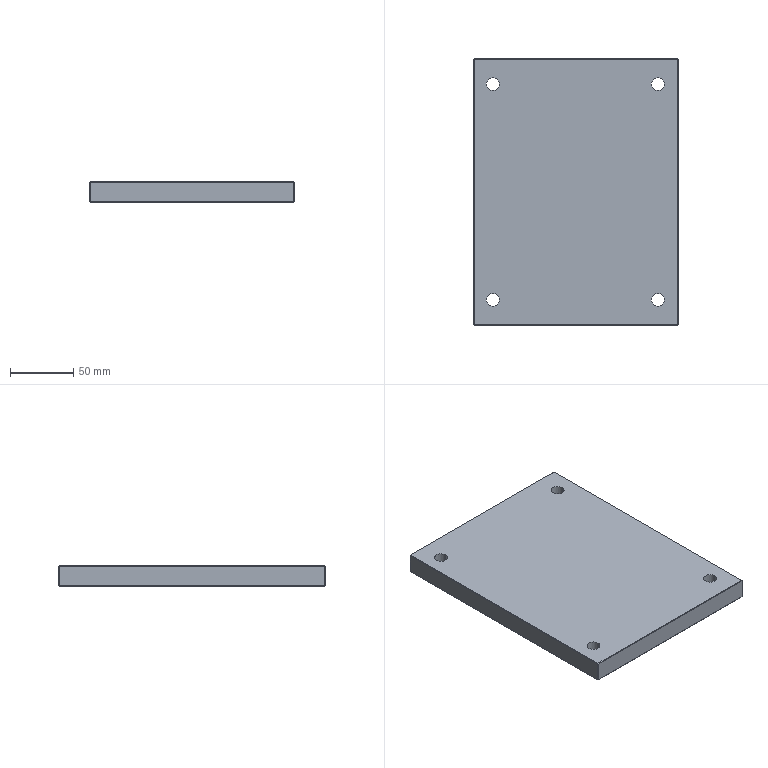Part | SolidWorks | features BaseBody 1 | 1 solid | 34 faces | box 161 x 210 x 16 mm | volume 535538 mm3 | plane 26 | cylinder 8 | commonest cylinder face diameters 10.2 x8
STEP:
#1=CARTESIAN_POINT('',(-15.1,290.,331.));
#2=VERTEX_POINT('',#1);
#3=CARTESIAN_POINT('',(-4.9,290.,331.));
#4=VERTEX_POINT('',#3);
#5=CARTESIAN_POINT('',(-10.,290.,331.));
#6=DIRECTION('',(0.,0.,1.));
#7=DIRECTION('',(0.,-1.,0.));
#8=AXIS2_PLACEMENT_3D('',#5,#6,#7);
#9=CIRCLE('',#8,5.1);
#10=EDGE_CURVE('',#2,#4,#9,.T.);
#11=ORIENTED_EDGE('',*,*,#10,.T.);
#12=CARTESIAN_POINT('',(-4.9,290.,315.));
#13=VERTEX_POINT('',#12);
#14=CARTESIAN_POINT('',(-4.9,290.,315.));
#15=DIRECTION('',(0.,0.,-1.));
#16=VECTOR('',#15,1000.);
#17=LINE('',#14,#16);
#18=EDGE_CURVE('',#4,#13,#17,.T.);
#19=ORIENTED_EDGE('',*,*,#18,.T.);
#20=CARTESIAN_POINT('',(-15.1,290.,315.));
#21=VERTEX_POINT('',#20);
#22=CARTESIAN_POINT('',(-10.,290.,315.));
#23=DIRECTION('',(0.,0.,-1.));
#24=DIRECTION('',(-1.,0.,0.));
#25=AXIS2_PLACEMENT_3D('',#22,#23,#24);
#26=CIRCLE('',#25,5.1);
#27=EDGE_CURVE('',#13,#21,#26,.T.);
#28=ORIENTED_EDGE('',*,*,#27,.T.);
#29=CARTESIAN_POINT('',(-15.1,290.,315.));
#30=DIRECTION('',(0.,0.,-1.));
#31=VECTOR('',#30,1000.);
#32=LINE('',#29,#31);
#33=EDGE_CURVE('',#2,#21,#32,.T.);
#34=ORIENTED_EDGE('',*,*,#33,.F.);
#35=EDGE_LOOP('',(#11,#19,#28,#34));
#36=FACE_OUTER_BOUND('',#35,.T.);
#37=CARTESIAN_POINT('',(-10.,290.,315.));
#38=DIRECTION('',(0.,0.,-1.));
#39=DIRECTION('',(-1.,0.,0.));
#40=AXIS2_PLACEMENT_3D('',#37,#38,#39);
#41=CYLINDRICAL_SURFACE('',#40,5.1);
#42=ADVANCED_FACE('',(#36),#41,.F.);
#43=CARTESIAN_POINT('',(-15.1,460.,331.));
#44=VERTEX_POINT('',#43);
#45=CARTESIAN_POINT('',(-4.9,460.,331.));
#46=VERTEX_POINT('',#45);
#47=CARTESIAN_POINT('',(-10.,460.,331.));
#48=DIRECTION('',(0.,0.,1.));
#49=DIRECTION('',(0.,-1.,0.));
#50=AXIS2_PLACEMENT_3D('',#47,#48,#49);
#51=CIRCLE('',#50,5.1);
#52=EDGE_CURVE('',#44,#46,#51,.T.);
#53=ORIENTED_EDGE('',*,*,#52,.T.);
#54=CARTESIAN_POINT('',(-4.9,460.,315.));
#55=VERTEX_POINT('',#54);
#56=CARTESIAN_POINT('',(-4.9,460.,315.));
#57=DIRECTION('',(0.,0.,-1.));
#58=VECTOR('',#57,1000.);
#59=LINE('',#56,#58);
#60=EDGE_CURVE('',#46,#55,#59,.T.);
#61=ORIENTED_EDGE('',*,*,#60,.T.);
#62=CARTESIAN_POINT('',(-15.1,460.,315.));
#63=VERTEX_POINT('',#62);
#64=CARTESIAN_POINT('',(-10.,460.,315.));
#65=DIRECTION('',(0.,0.,-1.));
#66=DIRECTION('',(-1.,0.,0.));
#67=AXIS2_PLACEMENT_3D('',#64,#65,#66);
#68=CIRCLE('',#67,5.1);
#69=EDGE_CURVE('',#55,#63,#68,.T.);
#70=ORIENTED_EDGE('',*,*,#69,.T.);
#71=CARTESIAN_POINT('',(-15.1,460.,315.));
#72=DIRECTION('',(0.,0.,-1.));
#73=VECTOR('',#72,1000.);
#74=LINE('',#71,#73);
#75=EDGE_CURVE('',#44,#63,#74,.T.);
#76=ORIENTED_EDGE('',*,*,#75,.F.);
#77=EDGE_LOOP('',(#53,#61,#70,#76));
#78=FACE_OUTER_BOUND('',#77,.T.);
#79=CARTESIAN_POINT('',(-10.,460.,315.));
#80=DIRECTION('',(0.,0.,-1.));
#81=DIRECTION('',(-1.,0.,0.));
#82=AXIS2_PLACEMENT_3D('',#79,#80,#81);
#83=CYLINDRICAL_SURFACE('',#82,5.1);
#84=ADVANCED_FACE('',(#78),#83,.F.);
#85=CARTESIAN_POINT('',(114.9,290.,331.));
#86=VERTEX_POINT('',#85);
#87=CARTESIAN_POINT('',(125.1,290.,331.));
#88=VERTEX_POINT('',#87);
#89=CARTESIAN_POINT('',(120.,290.,331.));
#90=DIRECTION('',(0.,0.,1.));
#91=DIRECTION('',(0.,-1.,0.));
#92=AXIS2_PLACEMENT_3D('',#89,#90,#91);
#93=CIRCLE('',#92,5.1);
#94=EDGE_CURVE('',#86,#88,#93,.T.);
#95=ORIENTED_EDGE('',*,*,#94,.T.);
#96=CARTESIAN_POINT('',(125.1,290.,315.));
#97=VERTEX_POINT('',#96);
#98=CARTESIAN_POINT('',(125.1,290.,315.));
#99=DIRECTION('',(0.,0.,-1.));
#100=VECTOR('',#99,1000.);
#101=LINE('',#98,#100);
#102=EDGE_CURVE('',#88,#97,#101,.T.);
#103=ORIENTED_EDGE('',*,*,#102,.T.);
#104=CARTESIAN_POINT('',(114.9,290.,315.));
#105=VERTEX_POINT('',#104);
#106=CARTESIAN_POINT('',(120.,290.,315.));
#107=DIRECTION('',(0.,0.,-1.));
#108=DIRECTION('',(-1.,0.,0.));
#109=AXIS2_PLACEMENT_3D('',#106,#107,#108);
#110=CIRCLE('',#109,5.1);
#111=EDGE_CURVE('',#97,#105,#110,.T.);
#112=ORIENTED_EDGE('',*,*,#111,.T.);
#113=CARTESIAN_POINT('',(114.9,290.,315.));
#114=DIRECTION('',(0.,0.,-1.));
#115=VECTOR('',#114,1000.);
#116=LINE('',#113,#115);
#117=EDGE_CURVE('',#86,#105,#116,.T.);
#118=ORIENTED_EDGE('',*,*,#117,.F.);
#119=EDGE_LOOP('',(#95,#103,#112,#118));
#120=FACE_OUTER_BOUND('',#119,.T.);
#121=CARTESIAN_POINT('',(120.,290.,315.));
#122=DIRECTION('',(0.,0.,-1.));
#123=DIRECTION('',(-1.,0.,0.));
#124=AXIS2_PLACEMENT_3D('',#121,#122,#123);
#125=CYLINDRICAL_SURFACE('',#124,5.1);
#126=ADVANCED_FACE('',(#120),#125,.F.);
#127=CARTESIAN_POINT('',(114.9,460.,331.));
#128=VERTEX_POINT('',#127);
#129=CARTESIAN_POINT('',(125.1,460.,331.));
#130=VERTEX_POINT('',#129);
#131=CARTESIAN_POINT('',(120.,460.,331.));
#132=DIRECTION('',(0.,0.,1.));
#133=DIRECTION('',(0.,-1.,0.));
#134=AXIS2_PLACEMENT_3D('',#131,#132,#133);
#135=CIRCLE('',#134,5.1);
#136=EDGE_CURVE('',#128,#130,#135,.T.);
#137=ORIENTED_EDGE('',*,*,#136,.T.);
#138=CARTESIAN_POINT('',(125.1,460.,315.));
#139=VERTEX_POINT('',#138);
#140=CARTESIAN_POINT('',(125.1,460.,315.));
#141=DIRECTION('',(0.,0.,-1.));
#142=VECTOR('',#141,1000.);
#143=LINE('',#140,#142);
#144=EDGE_CURVE('',#130,#139,#143,.T.);
#145=ORIENTED_EDGE('',*,*,#144,.T.);
#146=CARTESIAN_POINT('',(114.9,460.,315.));
#147=VERTEX_POINT('',#146);
#148=CARTESIAN_POINT('',(120.,460.,315.));
#149=DIRECTION('',(0.,0.,-1.));
#150=DIRECTION('',(-1.,0.,0.));
#151=AXIS2_PLACEMENT_3D('',#148,#149,#150);
#152=CIRCLE('',#151,5.1);
#153=EDGE_CURVE('',#139,#147,#152,.T.);
#154=ORIENTED_EDGE('',*,*,#153,.T.);
#155=CARTESIAN_POINT('',(114.9,460.,315.));
#156=DIRECTION('',(0.,0.,-1.));
#157=VECTOR('',#156,1000.);
#158=LINE('',#155,#157);
#159=EDGE_CURVE('',#128,#147,#158,.T.);
#160=ORIENTED_EDGE('',*,*,#159,.F.);
#161=EDGE_LOOP('',(#137,#145,#154,#160));
#162=FACE_OUTER_BOUND('',#161,.T.);
#163=CARTESIAN_POINT('',(120.,460.,315.));
#164=DIRECTION('',(0.,0.,-1.));
#165=DIRECTION('',(-1.,0.,0.));
#166=AXIS2_PLACEMENT_3D('',#163,#164,#165);
#167=CYLINDRICAL_SURFACE('',#166,5.1);
#168=ADVANCED_FACE('',(#162),#167,.F.);
#169=CARTESIAN_POINT('',(-25.,270.5,330.5));
#170=VERTEX_POINT('',#169);
#171=CARTESIAN_POINT('',(-24.5,270.5,331.));
#172=VERTEX_POINT('',#171);
#173=CARTESIAN_POINT('',(-24.5,270.5,331.));
#174=DIRECTION('',(0.7071,0.,0.7071));
#175=VECTOR('',#174,1000.);
#176=LINE('',#173,#175);
#177=EDGE_CURVE('',#170,#172,#176,.T.);
#178=ORIENTED_EDGE('',*,*,#177,.T.);
#179=CARTESIAN_POINT('',(-24.5,479.5,331.));
#180=VERTEX_POINT('',#179);
#181=CARTESIAN_POINT('',(-24.5,270.,331.));
#182=DIRECTION('',(0.,-1.,0.));
#183=VECTOR('',#182,1000.);
#184=LINE('',#181,#183);
#185=EDGE_CURVE('',#180,#172,#184,.T.);
#186=ORIENTED_EDGE('',*,*,#185,.F.);
#187=CARTESIAN_POINT('',(-25.,479.5,330.5));
#188=VERTEX_POINT('',#187);
#189=CARTESIAN_POINT('',(-25.,479.5,330.5));
#190=DIRECTION('',(-0.7071,0.,-0.7071));
#191=VECTOR('',#190,1000.);
#192=LINE('',#189,#191);
#193=EDGE_CURVE('',#180,#188,#192,.T.);
#194=ORIENTED_EDGE('',*,*,#193,.T.);
#195=CARTESIAN_POINT('',(-25.,480.,330.5));
#196=DIRECTION('',(0.,1.,0.));
#197=VECTOR('',#196,1000.);
#198=LINE('',#195,#197);
#199=EDGE_CURVE('',#170,#188,#198,.T.);
#200=ORIENTED_EDGE('',*,*,#199,.F.);
#201=EDGE_LOOP('',(#178,#186,#194,#200));
#202=FACE_OUTER_BOUND('',#201,.T.);
#203=CARTESIAN_POINT('',(-25.,0.,330.5));
#204=DIRECTION('',(-0.7071,0.,0.7071));
#205=DIRECTION('',(0.,1.,0.));
#206=AXIS2_PLACEMENT_3D('',#203,#204,#205);
#207=PLANE('',#206);
#208=ADVANCED_FACE('',(#202),#207,.T.);
#209=CARTESIAN_POINT('',(-24.5,480.,330.5));
#210=VERTEX_POINT('',#209);
#211=CARTESIAN_POINT('',(-24.5,479.75,330.75));
#212=DIRECTION('',(0.,0.7071,-0.7071));
#213=VECTOR('',#212,1000.);
#214=LINE('',#211,#213);
#215=EDGE_CURVE('',#180,#210,#214,.T.);
#216=ORIENTED_EDGE('',*,*,#215,.T.);
#217=CARTESIAN_POINT('',(-25.,479.5,330.5));
#218=DIRECTION('',(-0.7071,-0.7071,0.));
#219=VECTOR('',#218,1000.);
#220=LINE('',#217,#219);
#221=EDGE_CURVE('',#210,#188,#220,.T.);
#222=ORIENTED_EDGE('',*,*,#221,.T.);
#223=ORIENTED_EDGE('',*,*,#193,.F.);
#224=EDGE_LOOP('',(#216,#222,#223));
#225=FACE_OUTER_BOUND('',#224,.T.);
#226=CARTESIAN_POINT('',(-25.,479.5,330.5));
#227=DIRECTION('',(-0.5774,0.5774,0.5774));
#228=DIRECTION('',(0.7071,0.,0.7071));
#229=AXIS2_PLACEMENT_3D('',#226,#227,#228);
#230=PLANE('',#229);
#231=ADVANCED_FACE('',(#225),#230,.T.);
#232=CARTESIAN_POINT('',(-24.5,270.,330.5));
#233=VERTEX_POINT('',#232);
#234=CARTESIAN_POINT('',(-24.75,270.25,330.5));
#235=DIRECTION('',(0.7071,-0.7071,0.));
#236=VECTOR('',#235,1000.);
#237=LINE('',#234,#236);
#238=EDGE_CURVE('',#170,#233,#237,.T.);
#239=ORIENTED_EDGE('',*,*,#238,.T.);
#240=CARTESIAN_POINT('',(-24.5,270.5,331.));
#241=DIRECTION('',(0.,0.7071,0.7071));
#242=VECTOR('',#241,1000.);
#243=LINE('',#240,#242);
#244=EDGE_CURVE('',#233,#172,#243,.T.);
#245=ORIENTED_EDGE('',*,*,#244,.T.);
#246=ORIENTED_EDGE('',*,*,#177,.F.);
#247=EDGE_LOOP('',(#239,#245,#246));
#248=FACE_OUTER_BOUND('',#247,.T.);
#249=CARTESIAN_POINT('',(-24.5,270.5,331.));
#250=DIRECTION('',(-0.5774,-0.5774,0.5774));
#251=DIRECTION('',(-0.7071,0.7071,0.));
#252=AXIS2_PLACEMENT_3D('',#249,#250,#251);
#253=PLANE('',#252);
#254=ADVANCED_FACE('',(#248),#253,.T.);
#255=CARTESIAN_POINT('',(135.5,479.5,331.));
#256=VERTEX_POINT('',#255);
#257=CARTESIAN_POINT('',(135.5,480.,330.5));
#258=VERTEX_POINT('',#257);
#259=CARTESIAN_POINT('',(135.5,479.5,331.));
#260=DIRECTION('',(0.,0.7071,-0.7071));
#261=VECTOR('',#260,1000.);
#262=LINE('',#259,#261);
#263=EDGE_CURVE('',#256,#258,#262,.T.);
#264=ORIENTED_EDGE('',*,*,#263,.T.);
#265=CARTESIAN_POINT('',(135.,480.,330.5));
#266=DIRECTION('',(1.,0.,0.));
#267=VECTOR('',#266,1000.);
#268=LINE('',#265,#267);
#269=EDGE_CURVE('',#210,#258,#268,.T.);
#270=ORIENTED_EDGE('',*,*,#269,.F.);
#271=ORIENTED_EDGE('',*,*,#215,.F.);
#272=CARTESIAN_POINT('',(135.,479.5,331.));
#273=DIRECTION('',(-1.,0.,0.));
#274=VECTOR('',#273,1000.);
#275=LINE('',#272,#274);
#276=EDGE_CURVE('',#256,#180,#275,.T.);
#277=ORIENTED_EDGE('',*,*,#276,.F.);
#278=EDGE_LOOP('',(#264,#270,#271,#277));
#279=FACE_OUTER_BOUND('',#278,.T.);
#280=CARTESIAN_POINT('',(135.,479.5,331.));
#281=DIRECTION('',(0.,-0.7071,-0.7071));
#282=DIRECTION('',(0.,-0.7071,0.7071));
#283=AXIS2_PLACEMENT_3D('',#280,#281,#282);
#284=PLANE('',#283);
#285=ADVANCED_FACE('',(#279),#284,.F.);
#286=CARTESIAN_POINT('',(-24.5,480.,315.5));
#287=VERTEX_POINT('',#286);
#288=CARTESIAN_POINT('',(-25.,479.5,315.5));
#289=VERTEX_POINT('',#288);
#290=CARTESIAN_POINT('',(-24.75,479.75,315.5));
#291=DIRECTION('',(-0.7071,-0.7071,0.));
#292=VECTOR('',#291,1000.);
#293=LINE('',#290,#292);
#294=EDGE_CURVE('',#287,#289,#293,.T.);
#295=ORIENTED_EDGE('',*,*,#294,.T.);
#296=CARTESIAN_POINT('',(-25.,479.5,315.));
#297=DIRECTION('',(0.,0.,-1.));
#298=VECTOR('',#297,1000.);
#299=LINE('',#296,#298);
#300=EDGE_CURVE('',#188,#289,#299,.T.);
#301=ORIENTED_EDGE('',*,*,#300,.F.);
#302=ORIENTED_EDGE('',*,*,#221,.F.);
#303=CARTESIAN_POINT('',(-24.5,480.,331.));
#304=DIRECTION('',(0.,0.,1.));
#305=VECTOR('',#304,1000.);
#306=LINE('',#303,#305);
#307=EDGE_CURVE('',#287,#210,#306,.T.);
#308=ORIENTED_EDGE('',*,*,#307,.F.);
#309=EDGE_LOOP('',(#295,#301,#302,#308));
#310=FACE_OUTER_BOUND('',#309,.T.);
#311=CARTESIAN_POINT('',(-25.,479.5,100.));
#312=DIRECTION('',(-0.7071,0.7071,0.));
#313=DIRECTION('',(0.,0.,1.));
#314=AXIS2_PLACEMENT_3D('',#311,#312,#313);
#315=PLANE('',#314);
#316=ADVANCED_FACE('',(#310),#315,.T.);
#317=CARTESIAN_POINT('',(-25.,270.5,315.5));
#318=VERTEX_POINT('',#317);
#319=CARTESIAN_POINT('',(-24.5,270.,315.5));
#320=VERTEX_POINT('',#319);
#321=CARTESIAN_POINT('',(-25.,270.5,315.5));
#322=DIRECTION('',(0.7071,-0.7071,0.));
#323=VECTOR('',#322,1000.);
#324=LINE('',#321,#323);
#325=EDGE_CURVE('',#318,#320,#324,.T.);
#326=ORIENTED_EDGE('',*,*,#325,.T.);
#327=CARTESIAN_POINT('',(-24.5,270.,315.));
#328=DIRECTION('',(0.,0.,-1.));
#329=VECTOR('',#328,1000.);
#330=LINE('',#327,#329);
#331=EDGE_CURVE('',#233,#320,#330,.T.);
#332=ORIENTED_EDGE('',*,*,#331,.F.);
#333=ORIENTED_EDGE('',*,*,#238,.F.);
#334=CARTESIAN_POINT('',(-25.,270.5,331.));
#335=DIRECTION('',(0.,0.,1.));
#336=VECTOR('',#335,1000.);
#337=LINE('',#334,#336);
#338=EDGE_CURVE('',#318,#170,#337,.T.);
#339=ORIENTED_EDGE('',*,*,#338,.F.);
#340=EDGE_LOOP('',(#326,#332,#333,#339));
#341=FACE_OUTER_BOUND('',#340,.T.);
#342=CARTESIAN_POINT('',(-25.,270.5,100.));
#343=DIRECTION('',(-0.7071,-0.7071,0.));
#344=DIRECTION('',(-0.7071,0.7071,0.));
#345=AXIS2_PLACEMENT_3D('',#342,#343,#344);
#346=PLANE('',#345);
#347=ADVANCED_FACE('',(#341),#346,.T.);
#348=CARTESIAN_POINT('',(135.5,270.,330.5));
#349=VERTEX_POINT('',#348);
#350=CARTESIAN_POINT('',(135.5,270.5,331.));
#351=VERTEX_POINT('',#350);
#352=CARTESIAN_POINT('',(135.5,270.5,331.));
#353=DIRECTION('',(0.,0.7071,0.7071));
#354=VECTOR('',#353,1000.);
#355=LINE('',#352,#354);
#356=EDGE_CURVE('',#349,#351,#355,.T.);
#357=ORIENTED_EDGE('',*,*,#356,.T.);
#358=CARTESIAN_POINT('',(135.,270.5,331.));
#359=DIRECTION('',(1.,0.,0.));
#360=VECTOR('',#359,1000.);
#361=LINE('',#358,#360);
#362=EDGE_CURVE('',#172,#351,#361,.T.);
#363=ORIENTED_EDGE('',*,*,#362,.F.);
#364=ORIENTED_EDGE('',*,*,#244,.F.);
#365=CARTESIAN_POINT('',(135.,270.,330.5));
#366=DIRECTION('',(-1.,0.,0.));
#367=VECTOR('',#366,1000.);
#368=LINE('',#365,#367);
#369=EDGE_CURVE('',#349,#233,#368,.T.);
#370=ORIENTED_EDGE('',*,*,#369,.F.);
#371=EDGE_LOOP('',(#357,#363,#364,#370));
#372=FACE_OUTER_BOUND('',#371,.T.);
#373=CARTESIAN_POINT('',(135.,270.,330.5));
#374=DIRECTION('',(0.,0.7071,-0.7071));
#375=DIRECTION('',(-1.,0.,0.));
#376=AXIS2_PLACEMENT_3D('',#373,#374,#375);
#377=PLANE('',#376);
#378=ADVANCED_FACE('',(#372),#377,.F.);
#379=CARTESIAN_POINT('',(136.,479.5,330.5));
#380=VERTEX_POINT('',#379);
#381=CARTESIAN_POINT('',(135.5,479.5,331.));
#382=DIRECTION('',(0.7071,0.,-0.7071));
#383=VECTOR('',#382,1000.);
#384=LINE('',#381,#383);
#385=EDGE_CURVE('',#256,#380,#384,.T.);
#386=ORIENTED_EDGE('',*,*,#385,.T.);
#387=CARTESIAN_POINT('',(135.75,479.75,330.5));
#388=DIRECTION('',(-0.7071,0.7071,0.));
#389=VECTOR('',#388,1000.);
#390=LINE('',#387,#389);
#391=EDGE_CURVE('',#380,#258,#390,.T.);
#392=ORIENTED_EDGE('',*,*,#391,.T.);
#393=ORIENTED_EDGE('',*,*,#263,.F.);
#394=EDGE_LOOP('',(#386,#392,#393));
#395=FACE_OUTER_BOUND('',#394,.T.);
#396=CARTESIAN_POINT('',(135.5,479.5,331.));
#397=DIRECTION('',(0.5774,0.5774,0.5774));
#398=DIRECTION('',(0.,0.7071,-0.7071));
#399=AXIS2_PLACEMENT_3D('',#396,#397,#398);
#400=PLANE('',#399);
#401=ADVANCED_FACE('',(#395),#400,.T.);
#402=CARTESIAN_POINT('',(-24.5,479.5,315.));
#403=VERTEX_POINT('',#402);
#404=CARTESIAN_POINT('',(-24.5,479.5,315.));
#405=DIRECTION('',(0.,-0.7071,-0.7071));
#406=VECTOR('',#405,1000.);
#407=LINE('',#404,#406);
#408=EDGE_CURVE('',#287,#403,#407,.T.);
#409=ORIENTED_EDGE('',*,*,#408,.T.);
#410=CARTESIAN_POINT('',(-24.5,479.5,315.));
#411=DIRECTION('',(-0.7071,0.,0.7071));
#412=VECTOR('',#411,1000.);
#413=LINE('',#410,#412);
#414=EDGE_CURVE('',#403,#289,#413,.T.);
#415=ORIENTED_EDGE('',*,*,#414,.T.);
#416=ORIENTED_EDGE('',*,*,#294,.F.);
#417=EDGE_LOOP('',(#409,#415,#416));
#418=FACE_OUTER_BOUND('',#417,.T.);
#419=CARTESIAN_POINT('',(-24.5,479.5,315.));
#420=DIRECTION('',(-0.5774,0.5774,-0.5774));
#421=DIRECTION('',(-0.7071,0.,0.7071));
#422=AXIS2_PLACEMENT_3D('',#419,#420,#421);
#423=PLANE('',#422);
#424=ADVANCED_FACE('',(#418),#423,.T.);
#425=CARTESIAN_POINT('',(-24.5,270.5,315.));
#426=VERTEX_POINT('',#425);
#427=CARTESIAN_POINT('',(-25.,270.5,315.5));
#428=DIRECTION('',(0.7071,0.,-0.7071));
#429=VECTOR('',#428,1000.);
#430=LINE('',#427,#429);
#431=EDGE_CURVE('',#318,#426,#430,.T.);
#432=ORIENTED_EDGE('',*,*,#431,.T.);
#433=CARTESIAN_POINT('',(-24.5,270.25,315.25));
#434=DIRECTION('',(0.,-0.7071,0.7071));
#435=VECTOR('',#434,1000.);
#436=LINE('',#433,#435);
#437=EDGE_CURVE('',#426,#320,#436,.T.);
#438=ORIENTED_EDGE('',*,*,#437,.T.);
#439=ORIENTED_EDGE('',*,*,#325,.F.);
#440=EDGE_LOOP('',(#432,#438,#439));
#441=FACE_OUTER_BOUND('',#440,.T.);
#442=CARTESIAN_POINT('',(-25.,270.5,315.5));
#443=DIRECTION('',(-0.5774,-0.5774,-0.5774));
#444=DIRECTION('',(0.,-0.7071,0.7071));
#445=AXIS2_PLACEMENT_3D('',#442,#443,#444);
#446=PLANE('',#445);
#447=ADVANCED_FACE('',(#441),#446,.T.);
#448=CARTESIAN_POINT('',(136.,270.5,330.5));
#449=VERTEX_POINT('',#448);
#450=CARTESIAN_POINT('',(135.75,270.25,330.5));
#451=DIRECTION('',(0.7071,0.7071,0.));
#452=VECTOR('',#451,1000.);
#453=LINE('',#450,#452);
#454=EDGE_CURVE('',#349,#449,#453,.T.);
#455=ORIENTED_EDGE('',*,*,#454,.T.);
#456=CARTESIAN_POINT('',(135.5,270.5,331.));
#457=DIRECTION('',(-0.7071,0.,0.7071));
#458=VECTOR('',#457,1000.);
#459=LINE('',#456,#458);
#460=EDGE_CURVE('',#449,#351,#459,.T.);
#461=ORIENTED_EDGE('',*,*,#460,.T.);
#462=ORIENTED_EDGE('',*,*,#356,.F.);
#463=EDGE_LOOP('',(#455,#461,#462));
#464=FACE_OUTER_BOUND('',#463,.T.);
#465=CARTESIAN_POINT('',(135.5,270.5,331.));
#466=DIRECTION('',(0.5774,-0.5774,0.5774));
#467=DIRECTION('',(0.,-0.7071,-0.7071));
#468=AXIS2_PLACEMENT_3D('',#465,#466,#467);
#469=PLANE('',#468);
#470=ADVANCED_FACE('',(#464),#469,.T.);
#471=ORIENTED_EDGE('',*,*,#460,.F.);
#472=CARTESIAN_POINT('',(136.,270.,330.5));
#473=DIRECTION('',(0.,-1.,0.));
#474=VECTOR('',#473,1000.);
#475=LINE('',#472,#474);
#476=EDGE_CURVE('',#380,#449,#475,.T.);
#477=ORIENTED_EDGE('',*,*,#476,.F.);
#478=ORIENTED_EDGE('',*,*,#385,.F.);
#479=CARTESIAN_POINT('',(135.5,480.,331.));
#480=DIRECTION('',(0.,1.,0.));
#481=VECTOR('',#480,1000.);
#482=LINE('',#479,#481);
#483=EDGE_CURVE('',#351,#256,#482,.T.);
#484=ORIENTED_EDGE('',*,*,#483,.F.);
#485=EDGE_LOOP('',(#471,#477,#478,#484));
#486=FACE_OUTER_BOUND('',#485,.T.);
#487=CARTESIAN_POINT('',(136.,750.,330.5));
#488=DIRECTION('',(0.7071,0.,0.7071));
#489=DIRECTION('',(0.,-1.,0.));
#490=AXIS2_PLACEMENT_3D('',#487,#488,#489);
#491=PLANE('',#490);
#492=ADVANCED_FACE('',(#486),#491,.T.);
#493=CARTESIAN_POINT('',(136.,479.5,315.5));
#494=VERTEX_POINT('',#493);
#495=CARTESIAN_POINT('',(135.5,480.,315.5));
#496=VERTEX_POINT('',#495);
#497=CARTESIAN_POINT('',(136.,479.5,315.5));
#498=DIRECTION('',(-0.7071,0.7071,0.));
#499=VECTOR('',#498,1000.);
#500=LINE('',#497,#499);
#501=EDGE_CURVE('',#494,#496,#500,.T.);
#502=ORIENTED_EDGE('',*,*,#501,.T.);
#503=CARTESIAN_POINT('',(135.5,480.,315.));
#504=DIRECTION('',(0.,0.,-1.));
#505=VECTOR('',#504,1000.);
#506=LINE('',#503,#505);
#507=EDGE_CURVE('',#258,#496,#506,.T.);
#508=ORIENTED_EDGE('',*,*,#507,.F.);
#509=ORIENTED_EDGE('',*,*,#391,.F.);
#510=CARTESIAN_POINT('',(136.,479.5,331.));
#511=DIRECTION('',(0.,0.,1.));
#512=VECTOR('',#511,1000.);
#513=LINE('',#510,#512);
#514=EDGE_CURVE('',#494,#380,#513,.T.);
#515=ORIENTED_EDGE('',*,*,#514,.F.);
#516=EDGE_LOOP('',(#502,#508,#509,#515));
#517=FACE_OUTER_BOUND('',#516,.T.);
#518=CARTESIAN_POINT('',(136.,479.5,333.));
#519=DIRECTION('',(0.7071,0.7071,0.));
#520=DIRECTION('',(0.,0.,-1.));
#521=AXIS2_PLACEMENT_3D('',#518,#519,#520);
#522=PLANE('',#521);
#523=ADVANCED_FACE('',(#517),#522,.T.);
#524=CARTESIAN_POINT('',(135.5,479.5,315.));
#525=VERTEX_POINT('',#524);
#526=CARTESIAN_POINT('',(135.5,479.75,315.25));
#527=DIRECTION('',(0.,-0.7071,-0.7071));
#528=VECTOR('',#527,1000.);
#529=LINE('',#526,#528);
#530=EDGE_CURVE('',#496,#525,#529,.T.);
#531=ORIENTED_EDGE('',*,*,#530,.T.);
#532=CARTESIAN_POINT('',(135.,479.5,315.));
#533=DIRECTION('',(1.,0.,0.));
#534=VECTOR('',#533,1000.);
#535=LINE('',#532,#534);
#536=EDGE_CURVE('',#403,#525,#535,.T.);
#537=ORIENTED_EDGE('',*,*,#536,.F.);
#538=ORIENTED_EDGE('',*,*,#408,.F.);
#539=CARTESIAN_POINT('',(135.,480.,315.5));
#540=DIRECTION('',(-1.,0.,0.));
#541=VECTOR('',#540,1000.);
#542=LINE('',#539,#541);
#543=EDGE_CURVE('',#496,#287,#542,.T.);
#544=ORIENTED_EDGE('',*,*,#543,.F.);
#545=EDGE_LOOP('',(#531,#537,#538,#544));
#546=FACE_OUTER_BOUND('',#545,.T.);
#547=CARTESIAN_POINT('',(135.,480.,315.5));
#548=DIRECTION('',(0.,-0.7071,0.7071));
#549=DIRECTION('',(-1.,0.,0.));
#550=AXIS2_PLACEMENT_3D('',#547,#548,#549);
#551=PLANE('',#550);
#552=ADVANCED_FACE('',(#546),#551,.F.);
#553=ORIENTED_EDGE('',*,*,#414,.F.);
#554=CARTESIAN_POINT('',(-24.5,480.,315.));
#555=DIRECTION('',(0.,1.,0.));
#556=VECTOR('',#555,1000.);
#557=LINE('',#554,#556);
#558=EDGE_CURVE('',#426,#403,#557,.T.);
#559=ORIENTED_EDGE('',*,*,#558,.F.);
#560=ORIENTED_EDGE('',*,*,#431,.F.);
#561=CARTESIAN_POINT('',(-25.,270.,315.5));
#562=DIRECTION('',(0.,-1.,0.));
#563=VECTOR('',#562,1000.);
#564=LINE('',#561,#563);
#565=EDGE_CURVE('',#289,#318,#564,.T.);
#566=ORIENTED_EDGE('',*,*,#565,.F.);
#567=EDGE_LOOP('',(#553,#559,#560,#566));
#568=FACE_OUTER_BOUND('',#567,.T.);
#569=CARTESIAN_POINT('',(-25.,0.,315.5));
#570=DIRECTION('',(-0.7071,0.,-0.7071));
#571=DIRECTION('',(-0.7071,0.,0.7071));
#572=AXIS2_PLACEMENT_3D('',#569,#570,#571);
#573=PLANE('',#572);
#574=ADVANCED_FACE('',(#568),#573,.T.);
#575=CARTESIAN_POINT('',(135.5,270.5,315.));
#576=VERTEX_POINT('',#575);
#577=CARTESIAN_POINT('',(135.5,270.,315.5));
#578=VERTEX_POINT('',#577);
#579=CARTESIAN_POINT('',(135.5,270.,315.5));
#580=DIRECTION('',(0.,-0.7071,0.7071));
#581=VECTOR('',#580,1000.);
#582=LINE('',#579,#581);
#583=EDGE_CURVE('',#576,#578,#582,.T.);
#584=ORIENTED_EDGE('',*,*,#583,.T.);
#585=CARTESIAN_POINT('',(135.,270.,315.5));
#586=DIRECTION('',(1.,0.,0.));
#587=VECTOR('',#586,1000.);
#588=LINE('',#585,#587);
#589=EDGE_CURVE('',#320,#578,#588,.T.);
#590=ORIENTED_EDGE('',*,*,#589,.F.);
#591=ORIENTED_EDGE('',*,*,#437,.F.);
#592=CARTESIAN_POINT('',(135.,270.5,315.));
#593=DIRECTION('',(-1.,0.,0.));
#594=VECTOR('',#593,1000.);
#595=LINE('',#592,#594);
#596=EDGE_CURVE('',#576,#426,#595,.T.);
#597=ORIENTED_EDGE('',*,*,#596,.F.);
#598=EDGE_LOOP('',(#584,#590,#591,#597));
#599=FACE_OUTER_BOUND('',#598,.T.);
#600=CARTESIAN_POINT('',(135.,270.5,315.));
#601=DIRECTION('',(0.,0.7071,0.7071));
#602=DIRECTION('',(1.,0.,0.));
#603=AXIS2_PLACEMENT_3D('',#600,#601,#602);
#604=PLANE('',#603);
#605=ADVANCED_FACE('',(#599),#604,.F.);
#606=CARTESIAN_POINT('',(136.,270.5,315.5));
#607=VERTEX_POINT('',#606);
#608=CARTESIAN_POINT('',(135.5,270.,315.5));
#609=DIRECTION('',(0.7071,0.7071,0.));
#610=VECTOR('',#609,1000.);
#611=LINE('',#608,#610);
#612=EDGE_CURVE('',#578,#607,#611,.T.);
#613=ORIENTED_EDGE('',*,*,#612,.T.);
#614=CARTESIAN_POINT('',(136.,270.5,315.));
#615=DIRECTION('',(0.,0.,-1.));
#616=VECTOR('',#615,1000.);
#617=LINE('',#614,#616);
#618=EDGE_CURVE('',#449,#607,#617,.T.);
#619=ORIENTED_EDGE('',*,*,#618,.F.);
#620=ORIENTED_EDGE('',*,*,#454,.F.);
#621=CARTESIAN_POINT('',(135.5,270.,331.));
#622=DIRECTION('',(0.,0.,1.));
#623=VECTOR('',#622,1000.);
#624=LINE('',#621,#623);
#625=EDGE_CURVE('',#578,#349,#624,.T.);
#626=ORIENTED_EDGE('',*,*,#625,.F.);
#627=EDGE_LOOP('',(#613,#619,#620,#626));
#628=FACE_OUTER_BOUND('',#627,.T.);
#629=CARTESIAN_POINT('',(136.,270.5,333.));
#630=DIRECTION('',(0.7071,-0.7071,0.));
#631=DIRECTION('',(0.,0.,-1.));
#632=AXIS2_PLACEMENT_3D('',#629,#630,#631);
#633=PLANE('',#632);
#634=ADVANCED_FACE('',(#628),#633,.T.);
#635=ORIENTED_EDGE('',*,*,#501,.F.);
#636=CARTESIAN_POINT('',(136.,479.5,315.5));
#637=DIRECTION('',(-0.7071,0.,-0.7071));
#638=VECTOR('',#637,1000.);
#639=LINE('',#636,#638);
#640=EDGE_CURVE('',#494,#525,#639,.T.);
#641=ORIENTED_EDGE('',*,*,#640,.T.);
#642=ORIENTED_EDGE('',*,*,#530,.F.);
#643=EDGE_LOOP('',(#635,#641,#642));
#644=FACE_OUTER_BOUND('',#643,.T.);
#645=CARTESIAN_POINT('',(136.,479.5,315.5));
#646=DIRECTION('',(0.5774,0.5774,-0.5774));
#647=DIRECTION('',(0.,-0.7071,-0.7071));
#648=AXIS2_PLACEMENT_3D('',#645,#646,#647);
#649=PLANE('',#648);
#650=ADVANCED_FACE('',(#644),#649,.T.);
#651=ORIENTED_EDGE('',*,*,#583,.F.);
#652=CARTESIAN_POINT('',(135.75,270.5,315.25));
#653=DIRECTION('',(0.7071,0.,0.7071));
#654=VECTOR('',#653,1000.);
#655=LINE('',#652,#654);
#656=EDGE_CURVE('',#576,#607,#655,.T.);
#657=ORIENTED_EDGE('',*,*,#656,.T.);
#658=ORIENTED_EDGE('',*,*,#612,.F.);
#659=EDGE_LOOP('',(#651,#657,#658));
#660=FACE_OUTER_BOUND('',#659,.T.);
#661=CARTESIAN_POINT('',(135.5,270.,315.5));
#662=DIRECTION('',(0.5774,-0.5774,-0.5774));
#663=DIRECTION('',(0.,-0.7071,0.7071));
#664=AXIS2_PLACEMENT_3D('',#661,#662,#663);
#665=PLANE('',#664);
#666=ADVANCED_FACE('',(#660),#665,.T.);
#667=ORIENTED_EDGE('',*,*,#656,.F.);
#668=CARTESIAN_POINT('',(135.5,270.,315.));
#669=DIRECTION('',(0.,-1.,0.));
#670=VECTOR('',#669,1000.);
#671=LINE('',#668,#670);
#672=EDGE_CURVE('',#525,#576,#671,.T.);
#673=ORIENTED_EDGE('',*,*,#672,.F.);
#674=ORIENTED_EDGE('',*,*,#640,.F.);
#675=CARTESIAN_POINT('',(136.,480.,315.5));
#676=DIRECTION('',(0.,1.,0.));
#677=VECTOR('',#676,1000.);
#678=LINE('',#675,#677);
#679=EDGE_CURVE('',#607,#494,#678,.T.);
#680=ORIENTED_EDGE('',*,*,#679,.F.);
#681=EDGE_LOOP('',(#667,#673,#674,#680));
#682=FACE_OUTER_BOUND('',#681,.T.);
#683=CARTESIAN_POINT('',(136.,750.,315.5));
#684=DIRECTION('',(0.7071,0.,-0.7071));
#685=DIRECTION('',(0.,-1.,0.));
#686=AXIS2_PLACEMENT_3D('',#683,#684,#685);
#687=PLANE('',#686);
#688=ADVANCED_FACE('',(#682),#687,.T.);
#689=ORIENTED_EDGE('',*,*,#476,.T.);
#690=ORIENTED_EDGE('',*,*,#618,.T.);
#691=ORIENTED_EDGE('',*,*,#679,.T.);
#692=ORIENTED_EDGE('',*,*,#514,.T.);
#693=EDGE_LOOP('',(#689,#690,#691,#692));
#694=FACE_OUTER_BOUND('',#693,.T.);
#695=CARTESIAN_POINT('',(136.,750.,333.));
#696=DIRECTION('',(-1.,0.,0.));
#697=DIRECTION('',(0.,0.,1.));
#698=AXIS2_PLACEMENT_3D('',#695,#696,#697);
#699=PLANE('',#698);
#700=ADVANCED_FACE('',(#694),#699,.F.);
#701=ORIENTED_EDGE('',*,*,#565,.T.);
#702=ORIENTED_EDGE('',*,*,#338,.T.);
#703=ORIENTED_EDGE('',*,*,#199,.T.);
#704=ORIENTED_EDGE('',*,*,#300,.T.);
#705=EDGE_LOOP('',(#701,#702,#703,#704));
#706=FACE_OUTER_BOUND('',#705,.T.);
#707=CARTESIAN_POINT('',(-25.,0.,100.));
#708=DIRECTION('',(1.,0.,0.));
#709=DIRECTION('',(0.,1.,0.));
#710=AXIS2_PLACEMENT_3D('',#707,#708,#709);
#711=PLANE('',#710);
#712=ADVANCED_FACE('',(#706),#711,.F.);
#713=ORIENTED_EDGE('',*,*,#625,.T.);
#714=ORIENTED_EDGE('',*,*,#369,.T.);
#715=ORIENTED_EDGE('',*,*,#331,.T.);
#716=ORIENTED_EDGE('',*,*,#589,.T.);
#717=EDGE_LOOP('',(#713,#714,#715,#716));
#718=FACE_OUTER_BOUND('',#717,.T.);
#719=CARTESIAN_POINT('',(135.,270.,341.));
#720=DIRECTION('',(0.,-1.,0.));
#721=DIRECTION('',(0.,0.,-1.));
#722=AXIS2_PLACEMENT_3D('',#719,#720,#721);
#723=PLANE('',#722);
#724=ADVANCED_FACE('',(#718),#723,.T.);
#725=ORIENTED_EDGE('',*,*,#136,.F.);
#726=CARTESIAN_POINT('',(120.,460.,331.));
#727=DIRECTION('',(0.,0.,1.));
#728=DIRECTION('',(0.,-1.,0.));
#729=AXIS2_PLACEMENT_3D('',#726,#727,#728);
#730=CIRCLE('',#729,5.1);
#731=EDGE_CURVE('',#130,#128,#730,.T.);
#732=ORIENTED_EDGE('',*,*,#731,.F.);
#733=EDGE_LOOP('',(#725,#732));
#734=FACE_BOUND('',#733,.T.);
#735=ORIENTED_EDGE('',*,*,#94,.F.);
#736=CARTESIAN_POINT('',(120.,290.,331.));
#737=DIRECTION('',(0.,0.,1.));
#738=DIRECTION('',(0.,-1.,0.));
#739=AXIS2_PLACEMENT_3D('',#736,#737,#738);
#740=CIRCLE('',#739,5.1);
#741=EDGE_CURVE('',#88,#86,#740,.T.);
#742=ORIENTED_EDGE('',*,*,#741,.F.);
#743=EDGE_LOOP('',(#735,#742));
#744=FACE_BOUND('',#743,.T.);
#745=ORIENTED_EDGE('',*,*,#52,.F.);
#746=CARTESIAN_POINT('',(-10.,460.,331.));
#747=DIRECTION('',(0.,0.,1.));
#748=DIRECTION('',(0.,-1.,0.));
#749=AXIS2_PLACEMENT_3D('',#746,#747,#748);
#750=CIRCLE('',#749,5.1);
#751=EDGE_CURVE('',#46,#44,#750,.T.);
#752=ORIENTED_EDGE('',*,*,#751,.F.);
#753=EDGE_LOOP('',(#745,#752));
#754=FACE_BOUND('',#753,.T.);
#755=ORIENTED_EDGE('',*,*,#10,.F.);
#756=CARTESIAN_POINT('',(-10.,290.,331.));
#757=DIRECTION('',(0.,0.,1.));
#758=DIRECTION('',(0.,-1.,0.));
#759=AXIS2_PLACEMENT_3D('',#756,#757,#758);
#760=CIRCLE('',#759,5.1);
#761=EDGE_CURVE('',#4,#2,#760,.T.);
#762=ORIENTED_EDGE('',*,*,#761,.F.);
#763=EDGE_LOOP('',(#755,#762));
#764=FACE_BOUND('',#763,.T.);
#765=ORIENTED_EDGE('',*,*,#276,.T.);
#766=ORIENTED_EDGE('',*,*,#185,.T.);
#767=ORIENTED_EDGE('',*,*,#362,.T.);
#768=ORIENTED_EDGE('',*,*,#483,.T.);
#769=EDGE_LOOP('',(#765,#766,#767,#768));
#770=FACE_OUTER_BOUND('',#769,.T.);
#771=CARTESIAN_POINT('',(135.,480.,331.));
#772=DIRECTION('',(0.,0.,1.));
#773=DIRECTION('',(0.,-1.,0.));
#774=AXIS2_PLACEMENT_3D('',#771,#772,#773);
#775=PLANE('',#774);
#776=ADVANCED_FACE('',(#734,#744,#754,#764,#770),#775,.T.);
#777=ORIENTED_EDGE('',*,*,#507,.T.);
#778=ORIENTED_EDGE('',*,*,#543,.T.);
#779=ORIENTED_EDGE('',*,*,#307,.T.);
#780=ORIENTED_EDGE('',*,*,#269,.T.);
#781=EDGE_LOOP('',(#777,#778,#779,#780));
#782=FACE_OUTER_BOUND('',#781,.T.);
#783=CARTESIAN_POINT('',(135.,480.,341.));
#784=DIRECTION('',(0.,1.,0.));
#785=DIRECTION('',(1.,0.,0.));
#786=AXIS2_PLACEMENT_3D('',#783,#784,#785);
#787=PLANE('',#786);
#788=ADVANCED_FACE('',(#782),#787,.T.);
#789=CARTESIAN_POINT('',(120.,460.,315.));
#790=DIRECTION('',(0.,0.,-1.));
#791=DIRECTION('',(-1.,0.,0.));
#792=AXIS2_PLACEMENT_3D('',#789,#790,#791);
#793=CIRCLE('',#792,5.1);
#794=EDGE_CURVE('',#147,#139,#793,.T.);
#795=ORIENTED_EDGE('',*,*,#794,.F.);
#796=ORIENTED_EDGE('',*,*,#153,.F.);
#797=EDGE_LOOP('',(#795,#796));
#798=FACE_BOUND('',#797,.T.);
#799=CARTESIAN_POINT('',(120.,290.,315.));
#800=DIRECTION('',(0.,0.,-1.));
#801=DIRECTION('',(-1.,0.,0.));
#802=AXIS2_PLACEMENT_3D('',#799,#800,#801);
#803=CIRCLE('',#802,5.1);
#804=EDGE_CURVE('',#105,#97,#803,.T.);
#805=ORIENTED_EDGE('',*,*,#804,.F.);
#806=ORIENTED_EDGE('',*,*,#111,.F.);
#807=EDGE_LOOP('',(#805,#806));
#808=FACE_BOUND('',#807,.T.);
#809=CARTESIAN_POINT('',(-10.,460.,315.));
#810=DIRECTION('',(0.,0.,-1.));
#811=DIRECTION('',(-1.,0.,0.));
#812=AXIS2_PLACEMENT_3D('',#809,#810,#811);
#813=CIRCLE('',#812,5.1);
#814=EDGE_CURVE('',#63,#55,#813,.T.);
#815=ORIENTED_EDGE('',*,*,#814,.F.);
#816=ORIENTED_EDGE('',*,*,#69,.F.);
#817=EDGE_LOOP('',(#815,#816));
#818=FACE_BOUND('',#817,.T.);
#819=CARTESIAN_POINT('',(-10.,290.,315.));
#820=DIRECTION('',(0.,0.,-1.));
#821=DIRECTION('',(-1.,0.,0.));
#822=AXIS2_PLACEMENT_3D('',#819,#820,#821);
#823=CIRCLE('',#822,5.1);
#824=EDGE_CURVE('',#21,#13,#823,.T.);
#825=ORIENTED_EDGE('',*,*,#824,.F.);
#826=ORIENTED_EDGE('',*,*,#27,.F.);
#827=EDGE_LOOP('',(#825,#826));
#828=FACE_BOUND('',#827,.T.);
#829=ORIENTED_EDGE('',*,*,#596,.T.);
#830=ORIENTED_EDGE('',*,*,#558,.T.);
#831=ORIENTED_EDGE('',*,*,#536,.T.);
#832=ORIENTED_EDGE('',*,*,#672,.T.);
#833=EDGE_LOOP('',(#829,#830,#831,#832));
#834=FACE_OUTER_BOUND('',#833,.T.);
#835=CARTESIAN_POINT('',(135.,480.,315.));
#836=DIRECTION('',(0.,0.,-1.));
#837=DIRECTION('',(0.,-1.,0.));
#838=AXIS2_PLACEMENT_3D('',#835,#836,#837);
#839=PLANE('',#838);
#840=ADVANCED_FACE('',(#798,#808,#818,#828,#834),#839,.T.);
#841=ORIENTED_EDGE('',*,*,#144,.F.);
#842=ORIENTED_EDGE('',*,*,#731,.T.);
#843=ORIENTED_EDGE('',*,*,#159,.T.);
#844=ORIENTED_EDGE('',*,*,#794,.T.);
#845=EDGE_LOOP('',(#841,#842,#843,#844));
#846=FACE_OUTER_BOUND('',#845,.T.);
#847=CARTESIAN_POINT('',(120.,460.,315.));
#848=DIRECTION('',(0.,0.,-1.));
#849=DIRECTION('',(-1.,0.,0.));
#850=AXIS2_PLACEMENT_3D('',#847,#848,#849);
#851=CYLINDRICAL_SURFACE('',#850,5.1);
#852=ADVANCED_FACE('',(#846),#851,.F.);
#853=ORIENTED_EDGE('',*,*,#102,.F.);
#854=ORIENTED_EDGE('',*,*,#741,.T.);
#855=ORIENTED_EDGE('',*,*,#117,.T.);
#856=ORIENTED_EDGE('',*,*,#804,.T.);
#857=EDGE_LOOP('',(#853,#854,#855,#856));
#858=FACE_OUTER_BOUND('',#857,.T.);
#859=CARTESIAN_POINT('',(120.,290.,315.));
#860=DIRECTION('',(0.,0.,-1.));
#861=DIRECTION('',(-1.,0.,0.));
#862=AXIS2_PLACEMENT_3D('',#859,#860,#861);
#863=CYLINDRICAL_SURFACE('',#862,5.1);
#864=ADVANCED_FACE('',(#858),#863,.F.);
#865=ORIENTED_EDGE('',*,*,#60,.F.);
#866=ORIENTED_EDGE('',*,*,#751,.T.);
#867=ORIENTED_EDGE('',*,*,#75,.T.);
#868=ORIENTED_EDGE('',*,*,#814,.T.);
#869=EDGE_LOOP('',(#865,#866,#867,#868));
#870=FACE_OUTER_BOUND('',#869,.T.);
#871=CARTESIAN_POINT('',(-10.,460.,315.));
#872=DIRECTION('',(0.,0.,-1.));
#873=DIRECTION('',(-1.,0.,0.));
#874=AXIS2_PLACEMENT_3D('',#871,#872,#873);
#875=CYLINDRICAL_SURFACE('',#874,5.1);
#876=ADVANCED_FACE('',(#870),#875,.F.);
#877=ORIENTED_EDGE('',*,*,#18,.F.);
#878=ORIENTED_EDGE('',*,*,#761,.T.);
#879=ORIENTED_EDGE('',*,*,#33,.T.);
#880=ORIENTED_EDGE('',*,*,#824,.T.);
#881=EDGE_LOOP('',(#877,#878,#879,#880));
#882=FACE_OUTER_BOUND('',#881,.T.);
#883=CARTESIAN_POINT('',(-10.,290.,315.));
#884=DIRECTION('',(0.,0.,-1.));
#885=DIRECTION('',(-1.,0.,0.));
#886=AXIS2_PLACEMENT_3D('',#883,#884,#885);
#887=CYLINDRICAL_SURFACE('',#886,5.1);
#888=ADVANCED_FACE('',(#882),#887,.F.);
#889=CLOSED_SHELL('',(#42,#84,#126,#168,#208,#231,#254,#285,#316,#347,#378,#401,#424,#447,#470,#492,#523,#552,#574,#605,#634,#650,#666,#688,#700,#712,#724,#776,#788,#840,#852,#864,#876,#888));
#890=MANIFOLD_SOLID_BREP('',#889);
#891=CARTESIAN_POINT('',(0.,0.,0.));
#892=DIRECTION('',(0.,0.,1.));
#893=DIRECTION('',(1.,0.,0.));
#894=AXIS2_PLACEMENT_3D('',#891,#892,#893);
#895=(LENGTH_UNIT()NAMED_UNIT(*)SI_UNIT(.MILLI.,.METRE.));
#896=UNCERTAINTY_MEASURE_WITH_UNIT(LENGTH_MEASURE(0.00001),#895,'','');
#897=(NAMED_UNIT(*)PLANE_ANGLE_UNIT()SI_UNIT($,.RADIAN.));
#898=(NAMED_UNIT(*)SI_UNIT($,.STERADIAN.)SOLID_ANGLE_UNIT());
#899=(GEOMETRIC_REPRESENTATION_CONTEXT(3)GLOBAL_UNCERTAINTY_ASSIGNED_CONTEXT((#896))GLOBAL_UNIT_ASSIGNED_CONTEXT((#895,#897,#898))REPRESENTATION_CONTEXT('',''));
#900=ADVANCED_BREP_SHAPE_REPRESENTATION('',(#890,#894),#899);